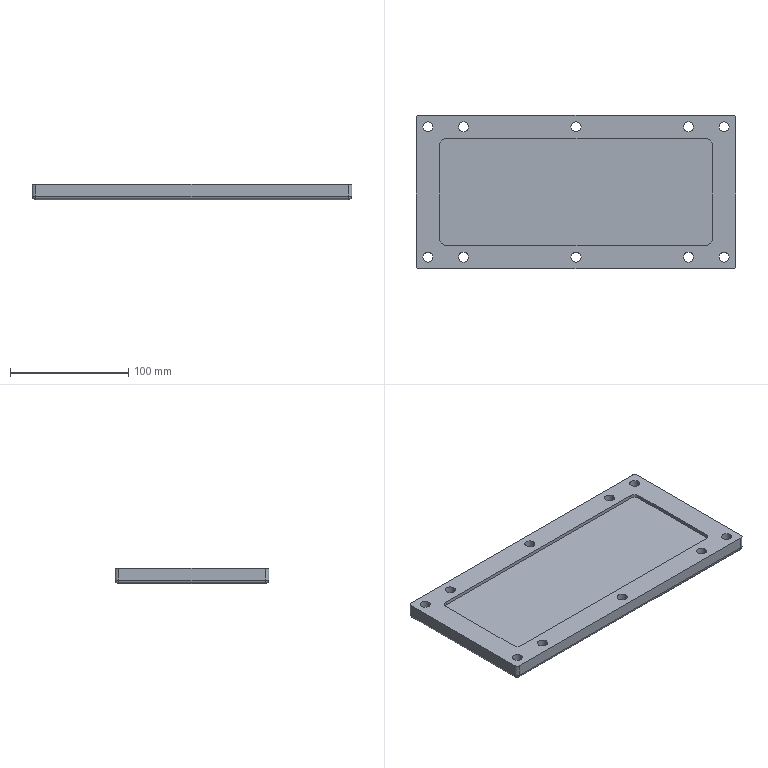Part | SolidWorks | features Extrusion 1, Fillet 1, ICE 1 | 1 solid | 47 faces | box 270 x 130 x 13 mm | volume 385260 mm3 | cylinder 32 | plane 11 | sphere 4 | commonest cylinder face diameters 8.5 x20 6 x8 10 x4
STEP:
#1=CARTESIAN_POINT('',(-129.25,-55.,13.));
#2=VERTEX_POINT('',#1);
#3=CARTESIAN_POINT('',(-120.75,-55.,13.));
#4=VERTEX_POINT('',#3);
#5=CARTESIAN_POINT('',(-125.,-55.,13.));
#6=DIRECTION('',(0.,0.,1.));
#7=DIRECTION('',(1.,0.,0.));
#8=AXIS2_PLACEMENT_3D('',#5,#6,#7);
#9=CIRCLE('',#8,4.25);
#10=EDGE_CURVE('',#2,#4,#9,.T.);
#11=ORIENTED_EDGE('',*,*,#10,.T.);
#12=CARTESIAN_POINT('',(-120.75,-55.,0.));
#13=VERTEX_POINT('',#12);
#14=CARTESIAN_POINT('',(-120.75,-55.,10.));
#15=DIRECTION('',(0.,0.,-1.));
#16=VECTOR('',#15,1000.);
#17=LINE('',#14,#16);
#18=EDGE_CURVE('',#4,#13,#17,.T.);
#19=ORIENTED_EDGE('',*,*,#18,.T.);
#20=CARTESIAN_POINT('',(-129.25,-55.,0.));
#21=VERTEX_POINT('',#20);
#22=CARTESIAN_POINT('',(-125.,-55.,0.));
#23=DIRECTION('',(0.,0.,1.));
#24=DIRECTION('',(1.,0.,0.));
#25=AXIS2_PLACEMENT_3D('',#22,#23,#24);
#26=CIRCLE('',#25,4.25);
#27=EDGE_CURVE('',#21,#13,#26,.T.);
#28=ORIENTED_EDGE('',*,*,#27,.F.);
#29=CARTESIAN_POINT('',(-129.25,-55.,10.));
#30=DIRECTION('',(0.,0.,-1.));
#31=VECTOR('',#30,1000.);
#32=LINE('',#29,#31);
#33=EDGE_CURVE('',#2,#21,#32,.T.);
#34=ORIENTED_EDGE('',*,*,#33,.F.);
#35=EDGE_LOOP('',(#11,#19,#28,#34));
#36=FACE_OUTER_BOUND('',#35,.T.);
#37=CARTESIAN_POINT('',(-125.,-55.,10.));
#38=DIRECTION('',(0.,0.,-1.));
#39=DIRECTION('',(-1.,0.,0.));
#40=AXIS2_PLACEMENT_3D('',#37,#38,#39);
#41=CYLINDRICAL_SURFACE('',#40,4.25);
#42=ADVANCED_FACE('',(#36),#41,.F.);
#43=CARTESIAN_POINT('',(-99.25,-55.,13.));
#44=VERTEX_POINT('',#43);
#45=CARTESIAN_POINT('',(-90.75,-55.,13.));
#46=VERTEX_POINT('',#45);
#47=CARTESIAN_POINT('',(-95.,-55.,13.));
#48=DIRECTION('',(0.,0.,1.));
#49=DIRECTION('',(1.,0.,0.));
#50=AXIS2_PLACEMENT_3D('',#47,#48,#49);
#51=CIRCLE('',#50,4.25);
#52=EDGE_CURVE('',#44,#46,#51,.T.);
#53=ORIENTED_EDGE('',*,*,#52,.T.);
#54=CARTESIAN_POINT('',(-90.75,-55.,0.));
#55=VERTEX_POINT('',#54);
#56=CARTESIAN_POINT('',(-90.75,-55.,10.));
#57=DIRECTION('',(0.,0.,-1.));
#58=VECTOR('',#57,1000.);
#59=LINE('',#56,#58);
#60=EDGE_CURVE('',#46,#55,#59,.T.);
#61=ORIENTED_EDGE('',*,*,#60,.T.);
#62=CARTESIAN_POINT('',(-99.25,-55.,0.));
#63=VERTEX_POINT('',#62);
#64=CARTESIAN_POINT('',(-95.,-55.,0.));
#65=DIRECTION('',(0.,0.,1.));
#66=DIRECTION('',(1.,0.,0.));
#67=AXIS2_PLACEMENT_3D('',#64,#65,#66);
#68=CIRCLE('',#67,4.25);
#69=EDGE_CURVE('',#63,#55,#68,.T.);
#70=ORIENTED_EDGE('',*,*,#69,.F.);
#71=CARTESIAN_POINT('',(-99.25,-55.,10.));
#72=DIRECTION('',(0.,0.,-1.));
#73=VECTOR('',#72,1000.);
#74=LINE('',#71,#73);
#75=EDGE_CURVE('',#44,#63,#74,.T.);
#76=ORIENTED_EDGE('',*,*,#75,.F.);
#77=EDGE_LOOP('',(#53,#61,#70,#76));
#78=FACE_OUTER_BOUND('',#77,.T.);
#79=CARTESIAN_POINT('',(-95.,-55.,10.));
#80=DIRECTION('',(0.,0.,-1.));
#81=DIRECTION('',(-1.,0.,0.));
#82=AXIS2_PLACEMENT_3D('',#79,#80,#81);
#83=CYLINDRICAL_SURFACE('',#82,4.25);
#84=ADVANCED_FACE('',(#78),#83,.F.);
#85=CARTESIAN_POINT('',(-4.25,-55.,13.));
#86=VERTEX_POINT('',#85);
#87=CARTESIAN_POINT('',(4.25,-55.,13.));
#88=VERTEX_POINT('',#87);
#89=CARTESIAN_POINT('',(0.,-55.,13.));
#90=DIRECTION('',(0.,0.,1.));
#91=DIRECTION('',(1.,0.,0.));
#92=AXIS2_PLACEMENT_3D('',#89,#90,#91);
#93=CIRCLE('',#92,4.25);
#94=EDGE_CURVE('',#86,#88,#93,.T.);
#95=ORIENTED_EDGE('',*,*,#94,.T.);
#96=CARTESIAN_POINT('',(4.25,-55.,0.));
#97=VERTEX_POINT('',#96);
#98=CARTESIAN_POINT('',(4.25,-55.,10.));
#99=DIRECTION('',(0.,0.,-1.));
#100=VECTOR('',#99,1000.);
#101=LINE('',#98,#100);
#102=EDGE_CURVE('',#88,#97,#101,.T.);
#103=ORIENTED_EDGE('',*,*,#102,.T.);
#104=CARTESIAN_POINT('',(-4.25,-55.,0.));
#105=VERTEX_POINT('',#104);
#106=CARTESIAN_POINT('',(0.,-55.,0.));
#107=DIRECTION('',(0.,0.,1.));
#108=DIRECTION('',(1.,0.,0.));
#109=AXIS2_PLACEMENT_3D('',#106,#107,#108);
#110=CIRCLE('',#109,4.25);
#111=EDGE_CURVE('',#105,#97,#110,.T.);
#112=ORIENTED_EDGE('',*,*,#111,.F.);
#113=CARTESIAN_POINT('',(-4.25,-55.,10.));
#114=DIRECTION('',(0.,0.,-1.));
#115=VECTOR('',#114,1000.);
#116=LINE('',#113,#115);
#117=EDGE_CURVE('',#86,#105,#116,.T.);
#118=ORIENTED_EDGE('',*,*,#117,.F.);
#119=EDGE_LOOP('',(#95,#103,#112,#118));
#120=FACE_OUTER_BOUND('',#119,.T.);
#121=CARTESIAN_POINT('',(0.,-55.,10.));
#122=DIRECTION('',(0.,0.,-1.));
#123=DIRECTION('',(-1.,0.,0.));
#124=AXIS2_PLACEMENT_3D('',#121,#122,#123);
#125=CYLINDRICAL_SURFACE('',#124,4.25);
#126=ADVANCED_FACE('',(#120),#125,.F.);
#127=CARTESIAN_POINT('',(90.75,-55.,13.));
#128=VERTEX_POINT('',#127);
#129=CARTESIAN_POINT('',(99.25,-55.,13.));
#130=VERTEX_POINT('',#129);
#131=CARTESIAN_POINT('',(95.,-55.,13.));
#132=DIRECTION('',(0.,0.,1.));
#133=DIRECTION('',(1.,0.,0.));
#134=AXIS2_PLACEMENT_3D('',#131,#132,#133);
#135=CIRCLE('',#134,4.25);
#136=EDGE_CURVE('',#128,#130,#135,.T.);
#137=ORIENTED_EDGE('',*,*,#136,.T.);
#138=CARTESIAN_POINT('',(99.25,-55.,0.));
#139=VERTEX_POINT('',#138);
#140=CARTESIAN_POINT('',(99.25,-55.,10.));
#141=DIRECTION('',(0.,0.,-1.));
#142=VECTOR('',#141,1000.);
#143=LINE('',#140,#142);
#144=EDGE_CURVE('',#130,#139,#143,.T.);
#145=ORIENTED_EDGE('',*,*,#144,.T.);
#146=CARTESIAN_POINT('',(90.75,-55.,0.));
#147=VERTEX_POINT('',#146);
#148=CARTESIAN_POINT('',(95.,-55.,0.));
#149=DIRECTION('',(0.,0.,1.));
#150=DIRECTION('',(1.,0.,0.));
#151=AXIS2_PLACEMENT_3D('',#148,#149,#150);
#152=CIRCLE('',#151,4.25);
#153=EDGE_CURVE('',#147,#139,#152,.T.);
#154=ORIENTED_EDGE('',*,*,#153,.F.);
#155=CARTESIAN_POINT('',(90.75,-55.,10.));
#156=DIRECTION('',(0.,0.,-1.));
#157=VECTOR('',#156,1000.);
#158=LINE('',#155,#157);
#159=EDGE_CURVE('',#128,#147,#158,.T.);
#160=ORIENTED_EDGE('',*,*,#159,.F.);
#161=EDGE_LOOP('',(#137,#145,#154,#160));
#162=FACE_OUTER_BOUND('',#161,.T.);
#163=CARTESIAN_POINT('',(95.,-55.,10.));
#164=DIRECTION('',(0.,0.,-1.));
#165=DIRECTION('',(-1.,0.,0.));
#166=AXIS2_PLACEMENT_3D('',#163,#164,#165);
#167=CYLINDRICAL_SURFACE('',#166,4.25);
#168=ADVANCED_FACE('',(#162),#167,.F.);
#169=CARTESIAN_POINT('',(120.75,-55.,13.));
#170=VERTEX_POINT('',#169);
#171=CARTESIAN_POINT('',(129.25,-55.,13.));
#172=VERTEX_POINT('',#171);
#173=CARTESIAN_POINT('',(125.,-55.,13.));
#174=DIRECTION('',(0.,0.,1.));
#175=DIRECTION('',(1.,0.,0.));
#176=AXIS2_PLACEMENT_3D('',#173,#174,#175);
#177=CIRCLE('',#176,4.25);
#178=EDGE_CURVE('',#170,#172,#177,.T.);
#179=ORIENTED_EDGE('',*,*,#178,.T.);
#180=CARTESIAN_POINT('',(129.25,-55.,0.));
#181=VERTEX_POINT('',#180);
#182=CARTESIAN_POINT('',(129.25,-55.,10.));
#183=DIRECTION('',(0.,0.,-1.));
#184=VECTOR('',#183,1000.);
#185=LINE('',#182,#184);
#186=EDGE_CURVE('',#172,#181,#185,.T.);
#187=ORIENTED_EDGE('',*,*,#186,.T.);
#188=CARTESIAN_POINT('',(120.75,-55.,0.));
#189=VERTEX_POINT('',#188);
#190=CARTESIAN_POINT('',(125.,-55.,0.));
#191=DIRECTION('',(0.,0.,1.));
#192=DIRECTION('',(1.,0.,0.));
#193=AXIS2_PLACEMENT_3D('',#190,#191,#192);
#194=CIRCLE('',#193,4.25);
#195=EDGE_CURVE('',#189,#181,#194,.T.);
#196=ORIENTED_EDGE('',*,*,#195,.F.);
#197=CARTESIAN_POINT('',(120.75,-55.,10.));
#198=DIRECTION('',(0.,0.,-1.));
#199=VECTOR('',#198,1000.);
#200=LINE('',#197,#199);
#201=EDGE_CURVE('',#170,#189,#200,.T.);
#202=ORIENTED_EDGE('',*,*,#201,.F.);
#203=EDGE_LOOP('',(#179,#187,#196,#202));
#204=FACE_OUTER_BOUND('',#203,.T.);
#205=CARTESIAN_POINT('',(125.,-55.,10.));
#206=DIRECTION('',(0.,0.,-1.));
#207=DIRECTION('',(-1.,0.,0.));
#208=AXIS2_PLACEMENT_3D('',#205,#206,#207);
#209=CYLINDRICAL_SURFACE('',#208,4.25);
#210=ADVANCED_FACE('',(#204),#209,.F.);
#211=CARTESIAN_POINT('',(120.75,55.,13.));
#212=VERTEX_POINT('',#211);
#213=CARTESIAN_POINT('',(129.25,55.,13.));
#214=VERTEX_POINT('',#213);
#215=CARTESIAN_POINT('',(125.,55.,13.));
#216=DIRECTION('',(0.,0.,1.));
#217=DIRECTION('',(1.,0.,0.));
#218=AXIS2_PLACEMENT_3D('',#215,#216,#217);
#219=CIRCLE('',#218,4.25);
#220=EDGE_CURVE('',#212,#214,#219,.T.);
#221=ORIENTED_EDGE('',*,*,#220,.T.);
#222=CARTESIAN_POINT('',(129.25,55.,0.));
#223=VERTEX_POINT('',#222);
#224=CARTESIAN_POINT('',(129.25,55.,10.));
#225=DIRECTION('',(0.,0.,-1.));
#226=VECTOR('',#225,1000.);
#227=LINE('',#224,#226);
#228=EDGE_CURVE('',#214,#223,#227,.T.);
#229=ORIENTED_EDGE('',*,*,#228,.T.);
#230=CARTESIAN_POINT('',(120.75,55.,0.));
#231=VERTEX_POINT('',#230);
#232=CARTESIAN_POINT('',(125.,55.,0.));
#233=DIRECTION('',(0.,0.,1.));
#234=DIRECTION('',(1.,0.,0.));
#235=AXIS2_PLACEMENT_3D('',#232,#233,#234);
#236=CIRCLE('',#235,4.25);
#237=EDGE_CURVE('',#231,#223,#236,.T.);
#238=ORIENTED_EDGE('',*,*,#237,.F.);
#239=CARTESIAN_POINT('',(120.75,55.,10.));
#240=DIRECTION('',(0.,0.,-1.));
#241=VECTOR('',#240,1000.);
#242=LINE('',#239,#241);
#243=EDGE_CURVE('',#212,#231,#242,.T.);
#244=ORIENTED_EDGE('',*,*,#243,.F.);
#245=EDGE_LOOP('',(#221,#229,#238,#244));
#246=FACE_OUTER_BOUND('',#245,.T.);
#247=CARTESIAN_POINT('',(125.,55.,10.));
#248=DIRECTION('',(0.,0.,-1.));
#249=DIRECTION('',(-1.,0.,0.));
#250=AXIS2_PLACEMENT_3D('',#247,#248,#249);
#251=CYLINDRICAL_SURFACE('',#250,4.25);
#252=ADVANCED_FACE('',(#246),#251,.F.);
#253=CARTESIAN_POINT('',(90.75,55.,13.));
#254=VERTEX_POINT('',#253);
#255=CARTESIAN_POINT('',(99.25,55.,13.));
#256=VERTEX_POINT('',#255);
#257=CARTESIAN_POINT('',(95.,55.,13.));
#258=DIRECTION('',(0.,0.,1.));
#259=DIRECTION('',(1.,0.,0.));
#260=AXIS2_PLACEMENT_3D('',#257,#258,#259);
#261=CIRCLE('',#260,4.25);
#262=EDGE_CURVE('',#254,#256,#261,.T.);
#263=ORIENTED_EDGE('',*,*,#262,.T.);
#264=CARTESIAN_POINT('',(99.25,55.,0.));
#265=VERTEX_POINT('',#264);
#266=CARTESIAN_POINT('',(99.25,55.,10.));
#267=DIRECTION('',(0.,0.,-1.));
#268=VECTOR('',#267,1000.);
#269=LINE('',#266,#268);
#270=EDGE_CURVE('',#256,#265,#269,.T.);
#271=ORIENTED_EDGE('',*,*,#270,.T.);
#272=CARTESIAN_POINT('',(90.75,55.,0.));
#273=VERTEX_POINT('',#272);
#274=CARTESIAN_POINT('',(95.,55.,0.));
#275=DIRECTION('',(0.,0.,1.));
#276=DIRECTION('',(1.,0.,0.));
#277=AXIS2_PLACEMENT_3D('',#274,#275,#276);
#278=CIRCLE('',#277,4.25);
#279=EDGE_CURVE('',#273,#265,#278,.T.);
#280=ORIENTED_EDGE('',*,*,#279,.F.);
#281=CARTESIAN_POINT('',(90.75,55.,10.));
#282=DIRECTION('',(0.,0.,-1.));
#283=VECTOR('',#282,1000.);
#284=LINE('',#281,#283);
#285=EDGE_CURVE('',#254,#273,#284,.T.);
#286=ORIENTED_EDGE('',*,*,#285,.F.);
#287=EDGE_LOOP('',(#263,#271,#280,#286));
#288=FACE_OUTER_BOUND('',#287,.T.);
#289=CARTESIAN_POINT('',(95.,55.,10.));
#290=DIRECTION('',(0.,0.,-1.));
#291=DIRECTION('',(-1.,0.,0.));
#292=AXIS2_PLACEMENT_3D('',#289,#290,#291);
#293=CYLINDRICAL_SURFACE('',#292,4.25);
#294=ADVANCED_FACE('',(#288),#293,.F.);
#295=CARTESIAN_POINT('',(-4.25,55.,13.));
#296=VERTEX_POINT('',#295);
#297=CARTESIAN_POINT('',(4.25,55.,13.));
#298=VERTEX_POINT('',#297);
#299=CARTESIAN_POINT('',(0.,55.,13.));
#300=DIRECTION('',(0.,0.,1.));
#301=DIRECTION('',(1.,0.,0.));
#302=AXIS2_PLACEMENT_3D('',#299,#300,#301);
#303=CIRCLE('',#302,4.25);
#304=EDGE_CURVE('',#296,#298,#303,.T.);
#305=ORIENTED_EDGE('',*,*,#304,.T.);
#306=CARTESIAN_POINT('',(4.25,55.,0.));
#307=VERTEX_POINT('',#306);
#308=CARTESIAN_POINT('',(4.25,55.,10.));
#309=DIRECTION('',(0.,0.,-1.));
#310=VECTOR('',#309,1000.);
#311=LINE('',#308,#310);
#312=EDGE_CURVE('',#298,#307,#311,.T.);
#313=ORIENTED_EDGE('',*,*,#312,.T.);
#314=CARTESIAN_POINT('',(-4.25,55.,0.));
#315=VERTEX_POINT('',#314);
#316=CARTESIAN_POINT('',(0.,55.,0.));
#317=DIRECTION('',(0.,0.,1.));
#318=DIRECTION('',(1.,0.,0.));
#319=AXIS2_PLACEMENT_3D('',#316,#317,#318);
#320=CIRCLE('',#319,4.25);
#321=EDGE_CURVE('',#315,#307,#320,.T.);
#322=ORIENTED_EDGE('',*,*,#321,.F.);
#323=CARTESIAN_POINT('',(-4.25,55.,10.));
#324=DIRECTION('',(0.,0.,-1.));
#325=VECTOR('',#324,1000.);
#326=LINE('',#323,#325);
#327=EDGE_CURVE('',#296,#315,#326,.T.);
#328=ORIENTED_EDGE('',*,*,#327,.F.);
#329=EDGE_LOOP('',(#305,#313,#322,#328));
#330=FACE_OUTER_BOUND('',#329,.T.);
#331=CARTESIAN_POINT('',(0.,55.,10.));
#332=DIRECTION('',(0.,0.,-1.));
#333=DIRECTION('',(-1.,0.,0.));
#334=AXIS2_PLACEMENT_3D('',#331,#332,#333);
#335=CYLINDRICAL_SURFACE('',#334,4.25);
#336=ADVANCED_FACE('',(#330),#335,.F.);
#337=CARTESIAN_POINT('',(-99.25,55.,13.));
#338=VERTEX_POINT('',#337);
#339=CARTESIAN_POINT('',(-90.75,55.,13.));
#340=VERTEX_POINT('',#339);
#341=CARTESIAN_POINT('',(-95.,55.,13.));
#342=DIRECTION('',(0.,0.,1.));
#343=DIRECTION('',(1.,0.,0.));
#344=AXIS2_PLACEMENT_3D('',#341,#342,#343);
#345=CIRCLE('',#344,4.25);
#346=EDGE_CURVE('',#338,#340,#345,.T.);
#347=ORIENTED_EDGE('',*,*,#346,.T.);
#348=CARTESIAN_POINT('',(-90.75,55.,0.));
#349=VERTEX_POINT('',#348);
#350=CARTESIAN_POINT('',(-90.75,55.,10.));
#351=DIRECTION('',(0.,0.,-1.));
#352=VECTOR('',#351,1000.);
#353=LINE('',#350,#352);
#354=EDGE_CURVE('',#340,#349,#353,.T.);
#355=ORIENTED_EDGE('',*,*,#354,.T.);
#356=CARTESIAN_POINT('',(-99.25,55.,0.));
#357=VERTEX_POINT('',#356);
#358=CARTESIAN_POINT('',(-95.,55.,0.));
#359=DIRECTION('',(0.,0.,1.));
#360=DIRECTION('',(1.,0.,0.));
#361=AXIS2_PLACEMENT_3D('',#358,#359,#360);
#362=CIRCLE('',#361,4.25);
#363=EDGE_CURVE('',#357,#349,#362,.T.);
#364=ORIENTED_EDGE('',*,*,#363,.F.);
#365=CARTESIAN_POINT('',(-99.25,55.,10.));
#366=DIRECTION('',(0.,0.,-1.));
#367=VECTOR('',#366,1000.);
#368=LINE('',#365,#367);
#369=EDGE_CURVE('',#338,#357,#368,.T.);
#370=ORIENTED_EDGE('',*,*,#369,.F.);
#371=EDGE_LOOP('',(#347,#355,#364,#370));
#372=FACE_OUTER_BOUND('',#371,.T.);
#373=CARTESIAN_POINT('',(-95.,55.,10.));
#374=DIRECTION('',(0.,0.,-1.));
#375=DIRECTION('',(-1.,0.,0.));
#376=AXIS2_PLACEMENT_3D('',#373,#374,#375);
#377=CYLINDRICAL_SURFACE('',#376,4.25);
#378=ADVANCED_FACE('',(#372),#377,.F.);
#379=CARTESIAN_POINT('',(-129.25,55.,13.));
#380=VERTEX_POINT('',#379);
#381=CARTESIAN_POINT('',(-120.75,55.,13.));
#382=VERTEX_POINT('',#381);
#383=CARTESIAN_POINT('',(-125.,55.,13.));
#384=DIRECTION('',(0.,0.,1.));
#385=DIRECTION('',(1.,0.,0.));
#386=AXIS2_PLACEMENT_3D('',#383,#384,#385);
#387=CIRCLE('',#386,4.25);
#388=EDGE_CURVE('',#380,#382,#387,.T.);
#389=ORIENTED_EDGE('',*,*,#388,.T.);
#390=CARTESIAN_POINT('',(-120.75,55.,0.));
#391=VERTEX_POINT('',#390);
#392=CARTESIAN_POINT('',(-120.75,55.,10.));
#393=DIRECTION('',(0.,0.,-1.));
#394=VECTOR('',#393,1000.);
#395=LINE('',#392,#394);
#396=EDGE_CURVE('',#382,#391,#395,.T.);
#397=ORIENTED_EDGE('',*,*,#396,.T.);
#398=CARTESIAN_POINT('',(-129.25,55.,0.));
#399=VERTEX_POINT('',#398);
#400=CARTESIAN_POINT('',(-125.,55.,0.));
#401=DIRECTION('',(0.,0.,1.));
#402=DIRECTION('',(1.,0.,0.));
#403=AXIS2_PLACEMENT_3D('',#400,#401,#402);
#404=CIRCLE('',#403,4.25);
#405=EDGE_CURVE('',#399,#391,#404,.T.);
#406=ORIENTED_EDGE('',*,*,#405,.F.);
#407=CARTESIAN_POINT('',(-129.25,55.,10.));
#408=DIRECTION('',(0.,0.,-1.));
#409=VECTOR('',#408,1000.);
#410=LINE('',#407,#409);
#411=EDGE_CURVE('',#380,#399,#410,.T.);
#412=ORIENTED_EDGE('',*,*,#411,.F.);
#413=EDGE_LOOP('',(#389,#397,#406,#412));
#414=FACE_OUTER_BOUND('',#413,.T.);
#415=CARTESIAN_POINT('',(-125.,55.,10.));
#416=DIRECTION('',(0.,0.,-1.));
#417=DIRECTION('',(-1.,0.,0.));
#418=AXIS2_PLACEMENT_3D('',#415,#416,#417);
#419=CYLINDRICAL_SURFACE('',#418,4.25);
#420=ADVANCED_FACE('',(#414),#419,.F.);
#421=CARTESIAN_POINT('',(132.,62.,0.));
#422=VERTEX_POINT('',#421);
#423=CARTESIAN_POINT('',(132.,-62.,0.));
#424=VERTEX_POINT('',#423);
#425=CARTESIAN_POINT('',(132.,-62.,0.));
#426=DIRECTION('',(0.,-1.,0.));
#427=VECTOR('',#426,1000.);
#428=LINE('',#425,#427);
#429=EDGE_CURVE('',#422,#424,#428,.T.);
#430=ORIENTED_EDGE('',*,*,#429,.T.);
#431=CARTESIAN_POINT('',(-132.,-62.,0.));
#432=VERTEX_POINT('',#431);
#433=CARTESIAN_POINT('',(-132.,-62.,0.));
#434=DIRECTION('',(-1.,0.,0.));
#435=VECTOR('',#434,1000.);
#436=LINE('',#433,#435);
#437=EDGE_CURVE('',#424,#432,#436,.T.);
#438=ORIENTED_EDGE('',*,*,#437,.T.);
#439=CARTESIAN_POINT('',(-132.,62.,0.));
#440=VERTEX_POINT('',#439);
#441=CARTESIAN_POINT('',(-132.,62.,0.));
#442=DIRECTION('',(0.,1.,0.));
#443=VECTOR('',#442,1000.);
#444=LINE('',#441,#443);
#445=EDGE_CURVE('',#432,#440,#444,.T.);
#446=ORIENTED_EDGE('',*,*,#445,.T.);
#447=CARTESIAN_POINT('',(132.,62.,0.));
#448=DIRECTION('',(1.,0.,0.));
#449=VECTOR('',#448,1000.);
#450=LINE('',#447,#449);
#451=EDGE_CURVE('',#440,#422,#450,.T.);
#452=ORIENTED_EDGE('',*,*,#451,.T.);
#453=EDGE_LOOP('',(#430,#438,#446,#452));
#454=FACE_OUTER_BOUND('',#453,.T.);
#455=ORIENTED_EDGE('',*,*,#69,.T.);
#456=CARTESIAN_POINT('',(-95.,-55.,0.));
#457=DIRECTION('',(0.,0.,1.));
#458=DIRECTION('',(1.,0.,0.));
#459=AXIS2_PLACEMENT_3D('',#456,#457,#458);
#460=CIRCLE('',#459,4.25);
#461=EDGE_CURVE('',#55,#63,#460,.T.);
#462=ORIENTED_EDGE('',*,*,#461,.T.);
#463=EDGE_LOOP('',(#455,#462));
#464=FACE_BOUND('',#463,.T.);
#465=ORIENTED_EDGE('',*,*,#153,.T.);
#466=CARTESIAN_POINT('',(95.,-55.,0.));
#467=DIRECTION('',(0.,0.,1.));
#468=DIRECTION('',(1.,0.,0.));
#469=AXIS2_PLACEMENT_3D('',#466,#467,#468);
#470=CIRCLE('',#469,4.25);
#471=EDGE_CURVE('',#139,#147,#470,.T.);
#472=ORIENTED_EDGE('',*,*,#471,.T.);
#473=EDGE_LOOP('',(#465,#472));
#474=FACE_BOUND('',#473,.T.);
#475=ORIENTED_EDGE('',*,*,#237,.T.);
#476=CARTESIAN_POINT('',(125.,55.,0.));
#477=DIRECTION('',(0.,0.,1.));
#478=DIRECTION('',(1.,0.,0.));
#479=AXIS2_PLACEMENT_3D('',#476,#477,#478);
#480=CIRCLE('',#479,4.25);
#481=EDGE_CURVE('',#223,#231,#480,.T.);
#482=ORIENTED_EDGE('',*,*,#481,.T.);
#483=EDGE_LOOP('',(#475,#482));
#484=FACE_BOUND('',#483,.T.);
#485=ORIENTED_EDGE('',*,*,#321,.T.);
#486=CARTESIAN_POINT('',(0.,55.,0.));
#487=DIRECTION('',(0.,0.,1.));
#488=DIRECTION('',(1.,0.,0.));
#489=AXIS2_PLACEMENT_3D('',#486,#487,#488);
#490=CIRCLE('',#489,4.25);
#491=EDGE_CURVE('',#307,#315,#490,.T.);
#492=ORIENTED_EDGE('',*,*,#491,.T.);
#493=EDGE_LOOP('',(#485,#492));
#494=FACE_BOUND('',#493,.T.);
#495=ORIENTED_EDGE('',*,*,#405,.T.);
#496=CARTESIAN_POINT('',(-125.,55.,0.));
#497=DIRECTION('',(0.,0.,1.));
#498=DIRECTION('',(1.,0.,0.));
#499=AXIS2_PLACEMENT_3D('',#496,#497,#498);
#500=CIRCLE('',#499,4.25);
#501=EDGE_CURVE('',#391,#399,#500,.T.);
#502=ORIENTED_EDGE('',*,*,#501,.T.);
#503=EDGE_LOOP('',(#495,#502));
#504=FACE_BOUND('',#503,.T.);
#505=ORIENTED_EDGE('',*,*,#363,.T.);
#506=CARTESIAN_POINT('',(-95.,55.,0.));
#507=DIRECTION('',(0.,0.,1.));
#508=DIRECTION('',(1.,0.,0.));
#509=AXIS2_PLACEMENT_3D('',#506,#507,#508);
#510=CIRCLE('',#509,4.25);
#511=EDGE_CURVE('',#349,#357,#510,.T.);
#512=ORIENTED_EDGE('',*,*,#511,.T.);
#513=EDGE_LOOP('',(#505,#512));
#514=FACE_BOUND('',#513,.T.);
#515=ORIENTED_EDGE('',*,*,#279,.T.);
#516=CARTESIAN_POINT('',(95.,55.,0.));
#517=DIRECTION('',(0.,0.,1.));
#518=DIRECTION('',(1.,0.,0.));
#519=AXIS2_PLACEMENT_3D('',#516,#517,#518);
#520=CIRCLE('',#519,4.25);
#521=EDGE_CURVE('',#265,#273,#520,.T.);
#522=ORIENTED_EDGE('',*,*,#521,.T.);
#523=EDGE_LOOP('',(#515,#522));
#524=FACE_BOUND('',#523,.T.);
#525=ORIENTED_EDGE('',*,*,#195,.T.);
#526=CARTESIAN_POINT('',(125.,-55.,0.));
#527=DIRECTION('',(0.,0.,1.));
#528=DIRECTION('',(1.,0.,0.));
#529=AXIS2_PLACEMENT_3D('',#526,#527,#528);
#530=CIRCLE('',#529,4.25);
#531=EDGE_CURVE('',#181,#189,#530,.T.);
#532=ORIENTED_EDGE('',*,*,#531,.T.);
#533=EDGE_LOOP('',(#525,#532));
#534=FACE_BOUND('',#533,.T.);
#535=ORIENTED_EDGE('',*,*,#111,.T.);
#536=CARTESIAN_POINT('',(0.,-55.,0.));
#537=DIRECTION('',(0.,0.,1.));
#538=DIRECTION('',(1.,0.,0.));
#539=AXIS2_PLACEMENT_3D('',#536,#537,#538);
#540=CIRCLE('',#539,4.25);
#541=EDGE_CURVE('',#97,#105,#540,.T.);
#542=ORIENTED_EDGE('',*,*,#541,.T.);
#543=EDGE_LOOP('',(#535,#542));
#544=FACE_BOUND('',#543,.T.);
#545=ORIENTED_EDGE('',*,*,#27,.T.);
#546=CARTESIAN_POINT('',(-125.,-55.,0.));
#547=DIRECTION('',(0.,0.,1.));
#548=DIRECTION('',(1.,0.,0.));
#549=AXIS2_PLACEMENT_3D('',#546,#547,#548);
#550=CIRCLE('',#549,4.25);
#551=EDGE_CURVE('',#13,#21,#550,.T.);
#552=ORIENTED_EDGE('',*,*,#551,.T.);
#553=EDGE_LOOP('',(#545,#552));
#554=FACE_BOUND('',#553,.T.);
#555=CARTESIAN_POINT('',(132.,62.,0.));
#556=DIRECTION('',(0.,0.,-1.));
#557=DIRECTION('',(-1.,0.,0.));
#558=AXIS2_PLACEMENT_3D('',#555,#556,#557);
#559=PLANE('',#558);
#560=ADVANCED_FACE('',(#454,#464,#474,#484,#494,#504,#514,#524,#534,#544,#554),#559,.T.);
#561=CARTESIAN_POINT('',(135.,62.,13.));
#562=VERTEX_POINT('',#561);
#563=CARTESIAN_POINT('',(135.,62.,3.));
#564=VERTEX_POINT('',#563);
#565=CARTESIAN_POINT('',(135.,62.,10.));
#566=DIRECTION('',(0.,0.,-1.));
#567=VECTOR('',#566,1000.);
#568=LINE('',#565,#567);
#569=EDGE_CURVE('',#562,#564,#568,.T.);
#570=ORIENTED_EDGE('',*,*,#569,.T.);
#571=CARTESIAN_POINT('',(132.,65.,3.));
#572=VERTEX_POINT('',#571);
#573=CARTESIAN_POINT('',(132.,62.,3.));
#574=DIRECTION('',(0.,0.,1.));
#575=DIRECTION('',(-1.,0.,0.));
#576=AXIS2_PLACEMENT_3D('',#573,#574,#575);
#577=CIRCLE('',#576,3.);
#578=EDGE_CURVE('',#564,#572,#577,.T.);
#579=ORIENTED_EDGE('',*,*,#578,.T.);
#580=CARTESIAN_POINT('',(132.,65.,13.));
#581=VERTEX_POINT('',#580);
#582=CARTESIAN_POINT('',(132.,65.,10.));
#583=DIRECTION('',(0.,0.,-1.));
#584=VECTOR('',#583,1000.);
#585=LINE('',#582,#584);
#586=EDGE_CURVE('',#581,#572,#585,.T.);
#587=ORIENTED_EDGE('',*,*,#586,.F.);
#588=CARTESIAN_POINT('',(132.,62.,13.));
#589=DIRECTION('',(0.,0.,1.));
#590=DIRECTION('',(1.,0.,0.));
#591=AXIS2_PLACEMENT_3D('',#588,#589,#590);
#592=CIRCLE('',#591,3.);
#593=EDGE_CURVE('',#562,#581,#592,.T.);
#594=ORIENTED_EDGE('',*,*,#593,.F.);
#595=EDGE_LOOP('',(#570,#579,#587,#594));
#596=FACE_OUTER_BOUND('',#595,.T.);
#597=CARTESIAN_POINT('',(132.,62.,10.));
#598=DIRECTION('',(0.,0.,-1.));
#599=DIRECTION('',(-1.,0.,0.));
#600=AXIS2_PLACEMENT_3D('',#597,#598,#599);
#601=CYLINDRICAL_SURFACE('',#600,3.);
#602=ADVANCED_FACE('',(#596),#601,.T.);
#603=ORIENTED_EDGE('',*,*,#586,.T.);
#604=CARTESIAN_POINT('',(-132.,65.,3.));
#605=VERTEX_POINT('',#604);
#606=CARTESIAN_POINT('',(-132.,65.,3.));
#607=DIRECTION('',(-1.,0.,0.));
#608=VECTOR('',#607,1000.);
#609=LINE('',#606,#608);
#610=EDGE_CURVE('',#572,#605,#609,.T.);
#611=ORIENTED_EDGE('',*,*,#610,.T.);
#612=CARTESIAN_POINT('',(-132.,65.,13.));
#613=VERTEX_POINT('',#612);
#614=CARTESIAN_POINT('',(-132.,65.,10.));
#615=DIRECTION('',(0.,0.,-1.));
#616=VECTOR('',#615,1000.);
#617=LINE('',#614,#616);
#618=EDGE_CURVE('',#613,#605,#617,.T.);
#619=ORIENTED_EDGE('',*,*,#618,.F.);
#620=CARTESIAN_POINT('',(132.,65.,13.));
#621=DIRECTION('',(-1.,0.,0.));
#622=VECTOR('',#621,1000.);
#623=LINE('',#620,#622);
#624=EDGE_CURVE('',#581,#613,#623,.T.);
#625=ORIENTED_EDGE('',*,*,#624,.F.);
#626=EDGE_LOOP('',(#603,#611,#619,#625));
#627=FACE_OUTER_BOUND('',#626,.T.);
#628=CARTESIAN_POINT('',(-132.,65.,10.));
#629=DIRECTION('',(0.,-1.,0.));
#630=DIRECTION('',(0.,0.,-1.));
#631=AXIS2_PLACEMENT_3D('',#628,#629,#630);
#632=PLANE('',#631);
#633=ADVANCED_FACE('',(#627),#632,.F.);
#634=ORIENTED_EDGE('',*,*,#618,.T.);
#635=CARTESIAN_POINT('',(-135.,62.,3.));
#636=VERTEX_POINT('',#635);
#637=CARTESIAN_POINT('',(-132.,62.,3.));
#638=DIRECTION('',(0.,0.,1.));
#639=DIRECTION('',(-1.,0.,0.));
#640=AXIS2_PLACEMENT_3D('',#637,#638,#639);
#641=CIRCLE('',#640,3.);
#642=EDGE_CURVE('',#605,#636,#641,.T.);
#643=ORIENTED_EDGE('',*,*,#642,.T.);
#644=CARTESIAN_POINT('',(-135.,62.,13.));
#645=VERTEX_POINT('',#644);
#646=CARTESIAN_POINT('',(-135.,62.,10.));
#647=DIRECTION('',(0.,0.,-1.));
#648=VECTOR('',#647,1000.);
#649=LINE('',#646,#648);
#650=EDGE_CURVE('',#645,#636,#649,.T.);
#651=ORIENTED_EDGE('',*,*,#650,.F.);
#652=CARTESIAN_POINT('',(-132.,62.,13.));
#653=DIRECTION('',(0.,0.,1.));
#654=DIRECTION('',(1.,0.,0.));
#655=AXIS2_PLACEMENT_3D('',#652,#653,#654);
#656=CIRCLE('',#655,3.);
#657=EDGE_CURVE('',#613,#645,#656,.T.);
#658=ORIENTED_EDGE('',*,*,#657,.F.);
#659=EDGE_LOOP('',(#634,#643,#651,#658));
#660=FACE_OUTER_BOUND('',#659,.T.);
#661=CARTESIAN_POINT('',(-132.,62.,10.));
#662=DIRECTION('',(0.,0.,-1.));
#663=DIRECTION('',(-1.,0.,0.));
#664=AXIS2_PLACEMENT_3D('',#661,#662,#663);
#665=CYLINDRICAL_SURFACE('',#664,3.);
#666=ADVANCED_FACE('',(#660),#665,.T.);
#667=ORIENTED_EDGE('',*,*,#650,.T.);
#668=CARTESIAN_POINT('',(-135.,-62.,3.));
#669=VERTEX_POINT('',#668);
#670=CARTESIAN_POINT('',(-135.,-62.,3.));
#671=DIRECTION('',(0.,-1.,0.));
#672=VECTOR('',#671,1000.);
#673=LINE('',#670,#672);
#674=EDGE_CURVE('',#636,#669,#673,.T.);
#675=ORIENTED_EDGE('',*,*,#674,.T.);
#676=CARTESIAN_POINT('',(-135.,-62.,13.));
#677=VERTEX_POINT('',#676);
#678=CARTESIAN_POINT('',(-135.,-62.,10.));
#679=DIRECTION('',(0.,0.,-1.));
#680=VECTOR('',#679,1000.);
#681=LINE('',#678,#680);
#682=EDGE_CURVE('',#677,#669,#681,.T.);
#683=ORIENTED_EDGE('',*,*,#682,.F.);
#684=CARTESIAN_POINT('',(-135.,62.,13.));
#685=DIRECTION('',(0.,-1.,0.));
#686=VECTOR('',#685,1000.);
#687=LINE('',#684,#686);
#688=EDGE_CURVE('',#645,#677,#687,.T.);
#689=ORIENTED_EDGE('',*,*,#688,.F.);
#690=EDGE_LOOP('',(#667,#675,#683,#689));
#691=FACE_OUTER_BOUND('',#690,.T.);
#692=CARTESIAN_POINT('',(-135.,-62.,10.));
#693=DIRECTION('',(1.,0.,0.));
#694=DIRECTION('',(0.,0.,-1.));
#695=AXIS2_PLACEMENT_3D('',#692,#693,#694);
#696=PLANE('',#695);
#697=ADVANCED_FACE('',(#691),#696,.F.);
#698=ORIENTED_EDGE('',*,*,#682,.T.);
#699=CARTESIAN_POINT('',(-132.,-65.,3.));
#700=VERTEX_POINT('',#699);
#701=CARTESIAN_POINT('',(-132.,-62.,3.));
#702=DIRECTION('',(0.,0.,1.));
#703=DIRECTION('',(-1.,0.,0.));
#704=AXIS2_PLACEMENT_3D('',#701,#702,#703);
#705=CIRCLE('',#704,3.);
#706=EDGE_CURVE('',#669,#700,#705,.T.);
#707=ORIENTED_EDGE('',*,*,#706,.T.);
#708=CARTESIAN_POINT('',(-132.,-65.,13.));
#709=VERTEX_POINT('',#708);
#710=CARTESIAN_POINT('',(-132.,-65.,10.));
#711=DIRECTION('',(0.,0.,-1.));
#712=VECTOR('',#711,1000.);
#713=LINE('',#710,#712);
#714=EDGE_CURVE('',#709,#700,#713,.T.);
#715=ORIENTED_EDGE('',*,*,#714,.F.);
#716=CARTESIAN_POINT('',(-132.,-62.,13.));
#717=DIRECTION('',(0.,0.,1.));
#718=DIRECTION('',(1.,0.,0.));
#719=AXIS2_PLACEMENT_3D('',#716,#717,#718);
#720=CIRCLE('',#719,3.);
#721=EDGE_CURVE('',#677,#709,#720,.T.);
#722=ORIENTED_EDGE('',*,*,#721,.F.);
#723=EDGE_LOOP('',(#698,#707,#715,#722));
#724=FACE_OUTER_BOUND('',#723,.T.);
#725=CARTESIAN_POINT('',(-132.,-62.,10.));
#726=DIRECTION('',(0.,0.,-1.));
#727=DIRECTION('',(-1.,0.,0.));
#728=AXIS2_PLACEMENT_3D('',#725,#726,#727);
#729=CYLINDRICAL_SURFACE('',#728,3.);
#730=ADVANCED_FACE('',(#724),#729,.T.);
#731=ORIENTED_EDGE('',*,*,#714,.T.);
#732=CARTESIAN_POINT('',(132.,-65.,3.));
#733=VERTEX_POINT('',#732);
#734=CARTESIAN_POINT('',(132.,-65.,3.));
#735=DIRECTION('',(1.,0.,0.));
#736=VECTOR('',#735,1000.);
#737=LINE('',#734,#736);
#738=EDGE_CURVE('',#700,#733,#737,.T.);
#739=ORIENTED_EDGE('',*,*,#738,.T.);
#740=CARTESIAN_POINT('',(132.,-65.,13.));
#741=VERTEX_POINT('',#740);
#742=CARTESIAN_POINT('',(132.,-65.,10.));
#743=DIRECTION('',(0.,0.,-1.));
#744=VECTOR('',#743,1000.);
#745=LINE('',#742,#744);
#746=EDGE_CURVE('',#741,#733,#745,.T.);
#747=ORIENTED_EDGE('',*,*,#746,.F.);
#748=CARTESIAN_POINT('',(-132.,-65.,13.));
#749=DIRECTION('',(1.,0.,0.));
#750=VECTOR('',#749,1000.);
#751=LINE('',#748,#750);
#752=EDGE_CURVE('',#709,#741,#751,.T.);
#753=ORIENTED_EDGE('',*,*,#752,.F.);
#754=EDGE_LOOP('',(#731,#739,#747,#753));
#755=FACE_OUTER_BOUND('',#754,.T.);
#756=CARTESIAN_POINT('',(-132.,-65.,10.));
#757=DIRECTION('',(0.,1.,0.));
#758=DIRECTION('',(0.,0.,1.));
#759=AXIS2_PLACEMENT_3D('',#756,#757,#758);
#760=PLANE('',#759);
#761=ADVANCED_FACE('',(#755),#760,.F.);
#762=ORIENTED_EDGE('',*,*,#746,.T.);
#763=CARTESIAN_POINT('',(135.,-62.,3.));
#764=VERTEX_POINT('',#763);
#765=CARTESIAN_POINT('',(132.,-62.,3.));
#766=DIRECTION('',(0.,0.,1.));
#767=DIRECTION('',(-1.,0.,0.));
#768=AXIS2_PLACEMENT_3D('',#765,#766,#767);
#769=CIRCLE('',#768,3.);
#770=EDGE_CURVE('',#733,#764,#769,.T.);
#771=ORIENTED_EDGE('',*,*,#770,.T.);
#772=CARTESIAN_POINT('',(135.,-62.,13.));
#773=VERTEX_POINT('',#772);
#774=CARTESIAN_POINT('',(135.,-62.,10.));
#775=DIRECTION('',(0.,0.,-1.));
#776=VECTOR('',#775,1000.);
#777=LINE('',#774,#776);
#778=EDGE_CURVE('',#773,#764,#777,.T.);
#779=ORIENTED_EDGE('',*,*,#778,.F.);
#780=CARTESIAN_POINT('',(132.,-62.,13.));
#781=DIRECTION('',(0.,0.,1.));
#782=DIRECTION('',(1.,0.,0.));
#783=AXIS2_PLACEMENT_3D('',#780,#781,#782);
#784=CIRCLE('',#783,3.);
#785=EDGE_CURVE('',#741,#773,#784,.T.);
#786=ORIENTED_EDGE('',*,*,#785,.F.);
#787=EDGE_LOOP('',(#762,#771,#779,#786));
#788=FACE_OUTER_BOUND('',#787,.T.);
#789=CARTESIAN_POINT('',(132.,-62.,10.));
#790=DIRECTION('',(0.,0.,-1.));
#791=DIRECTION('',(-1.,0.,0.));
#792=AXIS2_PLACEMENT_3D('',#789,#790,#791);
#793=CYLINDRICAL_SURFACE('',#792,3.);
#794=ADVANCED_FACE('',(#788),#793,.T.);
#795=ORIENTED_EDGE('',*,*,#778,.T.);
#796=CARTESIAN_POINT('',(135.,62.,3.));
#797=DIRECTION('',(0.,1.,0.));
#798=VECTOR('',#797,1000.);
#799=LINE('',#796,#798);
#800=EDGE_CURVE('',#764,#564,#799,.T.);
#801=ORIENTED_EDGE('',*,*,#800,.T.);
#802=ORIENTED_EDGE('',*,*,#569,.F.);
#803=CARTESIAN_POINT('',(135.,-62.,13.));
#804=DIRECTION('',(0.,1.,0.));
#805=VECTOR('',#804,1000.);
#806=LINE('',#803,#805);
#807=EDGE_CURVE('',#773,#562,#806,.T.);
#808=ORIENTED_EDGE('',*,*,#807,.F.);
#809=EDGE_LOOP('',(#795,#801,#802,#808));
#810=FACE_OUTER_BOUND('',#809,.T.);
#811=CARTESIAN_POINT('',(135.,-62.,10.));
#812=DIRECTION('',(-1.,0.,0.));
#813=DIRECTION('',(0.,0.,1.));
#814=AXIS2_PLACEMENT_3D('',#811,#812,#813);
#815=PLANE('',#814);
#816=ADVANCED_FACE('',(#810),#815,.F.);
#817=ORIENTED_EDGE('',*,*,#396,.F.);
#818=CARTESIAN_POINT('',(-125.,55.,13.));
#819=DIRECTION('',(0.,0.,1.));
#820=DIRECTION('',(1.,0.,0.));
#821=AXIS2_PLACEMENT_3D('',#818,#819,#820);
#822=CIRCLE('',#821,4.25);
#823=EDGE_CURVE('',#382,#380,#822,.T.);
#824=ORIENTED_EDGE('',*,*,#823,.T.);
#825=ORIENTED_EDGE('',*,*,#411,.T.);
#826=ORIENTED_EDGE('',*,*,#501,.F.);
#827=EDGE_LOOP('',(#817,#824,#825,#826));
#828=FACE_OUTER_BOUND('',#827,.T.);
#829=CARTESIAN_POINT('',(-125.,55.,10.));
#830=DIRECTION('',(0.,0.,-1.));
#831=DIRECTION('',(-1.,0.,0.));
#832=AXIS2_PLACEMENT_3D('',#829,#830,#831);
#833=CYLINDRICAL_SURFACE('',#832,4.25);
#834=ADVANCED_FACE('',(#828),#833,.F.);
#835=ORIENTED_EDGE('',*,*,#354,.F.);
#836=CARTESIAN_POINT('',(-95.,55.,13.));
#837=DIRECTION('',(0.,0.,1.));
#838=DIRECTION('',(1.,0.,0.));
#839=AXIS2_PLACEMENT_3D('',#836,#837,#838);
#840=CIRCLE('',#839,4.25);
#841=EDGE_CURVE('',#340,#338,#840,.T.);
#842=ORIENTED_EDGE('',*,*,#841,.T.);
#843=ORIENTED_EDGE('',*,*,#369,.T.);
#844=ORIENTED_EDGE('',*,*,#511,.F.);
#845=EDGE_LOOP('',(#835,#842,#843,#844));
#846=FACE_OUTER_BOUND('',#845,.T.);
#847=CARTESIAN_POINT('',(-95.,55.,10.));
#848=DIRECTION('',(0.,0.,-1.));
#849=DIRECTION('',(-1.,0.,0.));
#850=AXIS2_PLACEMENT_3D('',#847,#848,#849);
#851=CYLINDRICAL_SURFACE('',#850,4.25);
#852=ADVANCED_FACE('',(#846),#851,.F.);
#853=ORIENTED_EDGE('',*,*,#312,.F.);
#854=CARTESIAN_POINT('',(0.,55.,13.));
#855=DIRECTION('',(0.,0.,1.));
#856=DIRECTION('',(1.,0.,0.));
#857=AXIS2_PLACEMENT_3D('',#854,#855,#856);
#858=CIRCLE('',#857,4.25);
#859=EDGE_CURVE('',#298,#296,#858,.T.);
#860=ORIENTED_EDGE('',*,*,#859,.T.);
#861=ORIENTED_EDGE('',*,*,#327,.T.);
#862=ORIENTED_EDGE('',*,*,#491,.F.);
#863=EDGE_LOOP('',(#853,#860,#861,#862));
#864=FACE_OUTER_BOUND('',#863,.T.);
#865=CARTESIAN_POINT('',(0.,55.,10.));
#866=DIRECTION('',(0.,0.,-1.));
#867=DIRECTION('',(-1.,0.,0.));
#868=AXIS2_PLACEMENT_3D('',#865,#866,#867);
#869=CYLINDRICAL_SURFACE('',#868,4.25);
#870=ADVANCED_FACE('',(#864),#869,.F.);
#871=ORIENTED_EDGE('',*,*,#270,.F.);
#872=CARTESIAN_POINT('',(95.,55.,13.));
#873=DIRECTION('',(0.,0.,1.));
#874=DIRECTION('',(1.,0.,0.));
#875=AXIS2_PLACEMENT_3D('',#872,#873,#874);
#876=CIRCLE('',#875,4.25);
#877=EDGE_CURVE('',#256,#254,#876,.T.);
#878=ORIENTED_EDGE('',*,*,#877,.T.);
#879=ORIENTED_EDGE('',*,*,#285,.T.);
#880=ORIENTED_EDGE('',*,*,#521,.F.);
#881=EDGE_LOOP('',(#871,#878,#879,#880));
#882=FACE_OUTER_BOUND('',#881,.T.);
#883=CARTESIAN_POINT('',(95.,55.,10.));
#884=DIRECTION('',(0.,0.,-1.));
#885=DIRECTION('',(-1.,0.,0.));
#886=AXIS2_PLACEMENT_3D('',#883,#884,#885);
#887=CYLINDRICAL_SURFACE('',#886,4.25);
#888=ADVANCED_FACE('',(#882),#887,.F.);
#889=ORIENTED_EDGE('',*,*,#228,.F.);
#890=CARTESIAN_POINT('',(125.,55.,13.));
#891=DIRECTION('',(0.,0.,1.));
#892=DIRECTION('',(1.,0.,0.));
#893=AXIS2_PLACEMENT_3D('',#890,#891,#892);
#894=CIRCLE('',#893,4.25);
#895=EDGE_CURVE('',#214,#212,#894,.T.);
#896=ORIENTED_EDGE('',*,*,#895,.T.);
#897=ORIENTED_EDGE('',*,*,#243,.T.);
#898=ORIENTED_EDGE('',*,*,#481,.F.);
#899=EDGE_LOOP('',(#889,#896,#897,#898));
#900=FACE_OUTER_BOUND('',#899,.T.);
#901=CARTESIAN_POINT('',(125.,55.,10.));
#902=DIRECTION('',(0.,0.,-1.));
#903=DIRECTION('',(-1.,0.,0.));
#904=AXIS2_PLACEMENT_3D('',#901,#902,#903);
#905=CYLINDRICAL_SURFACE('',#904,4.25);
#906=ADVANCED_FACE('',(#900),#905,.F.);
#907=ORIENTED_EDGE('',*,*,#186,.F.);
#908=CARTESIAN_POINT('',(125.,-55.,13.));
#909=DIRECTION('',(0.,0.,1.));
#910=DIRECTION('',(1.,0.,0.));
#911=AXIS2_PLACEMENT_3D('',#908,#909,#910);
#912=CIRCLE('',#911,4.25);
#913=EDGE_CURVE('',#172,#170,#912,.T.);
#914=ORIENTED_EDGE('',*,*,#913,.T.);
#915=ORIENTED_EDGE('',*,*,#201,.T.);
#916=ORIENTED_EDGE('',*,*,#531,.F.);
#917=EDGE_LOOP('',(#907,#914,#915,#916));
#918=FACE_OUTER_BOUND('',#917,.T.);
#919=CARTESIAN_POINT('',(125.,-55.,10.));
#920=DIRECTION('',(0.,0.,-1.));
#921=DIRECTION('',(-1.,0.,0.));
#922=AXIS2_PLACEMENT_3D('',#919,#920,#921);
#923=CYLINDRICAL_SURFACE('',#922,4.25);
#924=ADVANCED_FACE('',(#918),#923,.F.);
#925=ORIENTED_EDGE('',*,*,#144,.F.);
#926=CARTESIAN_POINT('',(95.,-55.,13.));
#927=DIRECTION('',(0.,0.,1.));
#928=DIRECTION('',(1.,0.,0.));
#929=AXIS2_PLACEMENT_3D('',#926,#927,#928);
#930=CIRCLE('',#929,4.25);
#931=EDGE_CURVE('',#130,#128,#930,.T.);
#932=ORIENTED_EDGE('',*,*,#931,.T.);
#933=ORIENTED_EDGE('',*,*,#159,.T.);
#934=ORIENTED_EDGE('',*,*,#471,.F.);
#935=EDGE_LOOP('',(#925,#932,#933,#934));
#936=FACE_OUTER_BOUND('',#935,.T.);
#937=CARTESIAN_POINT('',(95.,-55.,10.));
#938=DIRECTION('',(0.,0.,-1.));
#939=DIRECTION('',(-1.,0.,0.));
#940=AXIS2_PLACEMENT_3D('',#937,#938,#939);
#941=CYLINDRICAL_SURFACE('',#940,4.25);
#942=ADVANCED_FACE('',(#936),#941,.F.);
#943=ORIENTED_EDGE('',*,*,#102,.F.);
#944=CARTESIAN_POINT('',(0.,-55.,13.));
#945=DIRECTION('',(0.,0.,1.));
#946=DIRECTION('',(1.,0.,0.));
#947=AXIS2_PLACEMENT_3D('',#944,#945,#946);
#948=CIRCLE('',#947,4.25);
#949=EDGE_CURVE('',#88,#86,#948,.T.);
#950=ORIENTED_EDGE('',*,*,#949,.T.);
#951=ORIENTED_EDGE('',*,*,#117,.T.);
#952=ORIENTED_EDGE('',*,*,#541,.F.);
#953=EDGE_LOOP('',(#943,#950,#951,#952));
#954=FACE_OUTER_BOUND('',#953,.T.);
#955=CARTESIAN_POINT('',(0.,-55.,10.));
#956=DIRECTION('',(0.,0.,-1.));
#957=DIRECTION('',(-1.,0.,0.));
#958=AXIS2_PLACEMENT_3D('',#955,#956,#957);
#959=CYLINDRICAL_SURFACE('',#958,4.25);
#960=ADVANCED_FACE('',(#954),#959,.F.);
#961=ORIENTED_EDGE('',*,*,#60,.F.);
#962=CARTESIAN_POINT('',(-95.,-55.,13.));
#963=DIRECTION('',(0.,0.,1.));
#964=DIRECTION('',(1.,0.,0.));
#965=AXIS2_PLACEMENT_3D('',#962,#963,#964);
#966=CIRCLE('',#965,4.25);
#967=EDGE_CURVE('',#46,#44,#966,.T.);
#968=ORIENTED_EDGE('',*,*,#967,.T.);
#969=ORIENTED_EDGE('',*,*,#75,.T.);
#970=ORIENTED_EDGE('',*,*,#461,.F.);
#971=EDGE_LOOP('',(#961,#968,#969,#970));
#972=FACE_OUTER_BOUND('',#971,.T.);
#973=CARTESIAN_POINT('',(-95.,-55.,10.));
#974=DIRECTION('',(0.,0.,-1.));
#975=DIRECTION('',(-1.,0.,0.));
#976=AXIS2_PLACEMENT_3D('',#973,#974,#975);
#977=CYLINDRICAL_SURFACE('',#976,4.25);
#978=ADVANCED_FACE('',(#972),#977,.F.);
#979=ORIENTED_EDGE('',*,*,#18,.F.);
#980=CARTESIAN_POINT('',(-125.,-55.,13.));
#981=DIRECTION('',(0.,0.,1.));
#982=DIRECTION('',(1.,0.,0.));
#983=AXIS2_PLACEMENT_3D('',#980,#981,#982);
#984=CIRCLE('',#983,4.25);
#985=EDGE_CURVE('',#4,#2,#984,.T.);
#986=ORIENTED_EDGE('',*,*,#985,.T.);
#987=ORIENTED_EDGE('',*,*,#33,.T.);
#988=ORIENTED_EDGE('',*,*,#551,.F.);
#989=EDGE_LOOP('',(#979,#986,#987,#988));
#990=FACE_OUTER_BOUND('',#989,.T.);
#991=CARTESIAN_POINT('',(-125.,-55.,10.));
#992=DIRECTION('',(0.,0.,-1.));
#993=DIRECTION('',(-1.,0.,0.));
#994=AXIS2_PLACEMENT_3D('',#991,#992,#993);
#995=CYLINDRICAL_SURFACE('',#994,4.25);
#996=ADVANCED_FACE('',(#990),#995,.F.);
#997=ORIENTED_EDGE('',*,*,#346,.F.);
#998=ORIENTED_EDGE('',*,*,#841,.F.);
#999=EDGE_LOOP('',(#997,#998));
#1000=FACE_BOUND('',#999,.T.);
#1001=ORIENTED_EDGE('',*,*,#262,.F.);
#1002=ORIENTED_EDGE('',*,*,#877,.F.);
#1003=EDGE_LOOP('',(#1001,#1002));
#1004=FACE_BOUND('',#1003,.T.);
#1005=ORIENTED_EDGE('',*,*,#178,.F.);
#1006=ORIENTED_EDGE('',*,*,#913,.F.);
#1007=EDGE_LOOP('',(#1005,#1006));
#1008=FACE_BOUND('',#1007,.T.);
#1009=ORIENTED_EDGE('',*,*,#94,.F.);
#1010=ORIENTED_EDGE('',*,*,#949,.F.);
#1011=EDGE_LOOP('',(#1009,#1010));
#1012=FACE_BOUND('',#1011,.T.);
#1013=ORIENTED_EDGE('',*,*,#10,.F.);
#1014=ORIENTED_EDGE('',*,*,#985,.F.);
#1015=EDGE_LOOP('',(#1013,#1014));
#1016=FACE_BOUND('',#1015,.T.);
#1017=ORIENTED_EDGE('',*,*,#593,.T.);
#1018=ORIENTED_EDGE('',*,*,#624,.T.);
#1019=ORIENTED_EDGE('',*,*,#657,.T.);
#1020=ORIENTED_EDGE('',*,*,#688,.T.);
#1021=ORIENTED_EDGE('',*,*,#721,.T.);
#1022=ORIENTED_EDGE('',*,*,#752,.T.);
#1023=ORIENTED_EDGE('',*,*,#785,.T.);
#1024=ORIENTED_EDGE('',*,*,#807,.T.);
#1025=EDGE_LOOP('',(#1017,#1018,#1019,#1020,#1021,#1022,#1023,#1024));
#1026=FACE_OUTER_BOUND('',#1025,.T.);
#1027=ORIENTED_EDGE('',*,*,#52,.F.);
#1028=ORIENTED_EDGE('',*,*,#967,.F.);
#1029=EDGE_LOOP('',(#1027,#1028));
#1030=FACE_BOUND('',#1029,.T.);
#1031=ORIENTED_EDGE('',*,*,#136,.F.);
#1032=ORIENTED_EDGE('',*,*,#931,.F.);
#1033=EDGE_LOOP('',(#1031,#1032));
#1034=FACE_BOUND('',#1033,.T.);
#1035=ORIENTED_EDGE('',*,*,#220,.F.);
#1036=ORIENTED_EDGE('',*,*,#895,.F.);
#1037=EDGE_LOOP('',(#1035,#1036));
#1038=FACE_BOUND('',#1037,.T.);
#1039=ORIENTED_EDGE('',*,*,#304,.F.);
#1040=ORIENTED_EDGE('',*,*,#859,.F.);
#1041=EDGE_LOOP('',(#1039,#1040));
#1042=FACE_BOUND('',#1041,.T.);
#1043=ORIENTED_EDGE('',*,*,#388,.F.);
#1044=ORIENTED_EDGE('',*,*,#823,.F.);
#1045=EDGE_LOOP('',(#1043,#1044));
#1046=FACE_BOUND('',#1045,.T.);
#1047=CARTESIAN_POINT('',(110.,45.,13.));
#1048=VERTEX_POINT('',#1047);
#1049=CARTESIAN_POINT('',(-110.,45.,13.));
#1050=VERTEX_POINT('',#1049);
#1051=CARTESIAN_POINT('',(-110.,45.,13.));
#1052=DIRECTION('',(-1.,0.,0.));
#1053=VECTOR('',#1052,1000.);
#1054=LINE('',#1051,#1053);
#1055=EDGE_CURVE('',#1048,#1050,#1054,.T.);
#1056=ORIENTED_EDGE('',*,*,#1055,.F.);
#1057=CARTESIAN_POINT('',(115.,40.,13.));
#1058=VERTEX_POINT('',#1057);
#1059=CARTESIAN_POINT('',(110.,40.,13.));
#1060=DIRECTION('',(0.,0.,1.));
#1061=DIRECTION('',(-1.,0.,0.));
#1062=AXIS2_PLACEMENT_3D('',#1059,#1060,#1061);
#1063=CIRCLE('',#1062,5.);
#1064=EDGE_CURVE('',#1058,#1048,#1063,.T.);
#1065=ORIENTED_EDGE('',*,*,#1064,.F.);
#1066=CARTESIAN_POINT('',(115.,-40.,13.));
#1067=VERTEX_POINT('',#1066);
#1068=CARTESIAN_POINT('',(115.,-40.,13.));
#1069=DIRECTION('',(0.,1.,0.));
#1070=VECTOR('',#1069,1000.);
#1071=LINE('',#1068,#1070);
#1072=EDGE_CURVE('',#1067,#1058,#1071,.T.);
#1073=ORIENTED_EDGE('',*,*,#1072,.F.);
#1074=CARTESIAN_POINT('',(110.,-45.,13.));
#1075=VERTEX_POINT('',#1074);
#1076=CARTESIAN_POINT('',(110.,-40.,13.));
#1077=DIRECTION('',(0.,0.,1.));
#1078=DIRECTION('',(1.,0.,0.));
#1079=AXIS2_PLACEMENT_3D('',#1076,#1077,#1078);
#1080=CIRCLE('',#1079,5.);
#1081=EDGE_CURVE('',#1075,#1067,#1080,.T.);
#1082=ORIENTED_EDGE('',*,*,#1081,.F.);
#1083=CARTESIAN_POINT('',(-110.,-45.,13.));
#1084=VERTEX_POINT('',#1083);
#1085=CARTESIAN_POINT('',(-110.,-45.,13.));
#1086=DIRECTION('',(1.,0.,0.));
#1087=VECTOR('',#1086,1000.);
#1088=LINE('',#1085,#1087);
#1089=EDGE_CURVE('',#1084,#1075,#1088,.T.);
#1090=ORIENTED_EDGE('',*,*,#1089,.F.);
#1091=CARTESIAN_POINT('',(-115.,-40.,13.));
#1092=VERTEX_POINT('',#1091);
#1093=CARTESIAN_POINT('',(-110.,-40.,13.));
#1094=DIRECTION('',(0.,0.,1.));
#1095=DIRECTION('',(1.,0.,0.));
#1096=AXIS2_PLACEMENT_3D('',#1093,#1094,#1095);
#1097=CIRCLE('',#1096,5.);
#1098=EDGE_CURVE('',#1092,#1084,#1097,.T.);
#1099=ORIENTED_EDGE('',*,*,#1098,.F.);
#1100=CARTESIAN_POINT('',(-115.,40.,13.));
#1101=VERTEX_POINT('',#1100);
#1102=CARTESIAN_POINT('',(-115.,-40.,13.));
#1103=DIRECTION('',(0.,-1.,0.));
#1104=VECTOR('',#1103,1000.);
#1105=LINE('',#1102,#1104);
#1106=EDGE_CURVE('',#1101,#1092,#1105,.T.);
#1107=ORIENTED_EDGE('',*,*,#1106,.F.);
#1108=CARTESIAN_POINT('',(-110.,40.,13.));
#1109=DIRECTION('',(0.,0.,1.));
#1110=DIRECTION('',(-1.,0.,0.));
#1111=AXIS2_PLACEMENT_3D('',#1108,#1109,#1110);
#1112=CIRCLE('',#1111,5.);
#1113=EDGE_CURVE('',#1050,#1101,#1112,.T.);
#1114=ORIENTED_EDGE('',*,*,#1113,.F.);
#1115=EDGE_LOOP('',(#1056,#1065,#1073,#1082,#1090,#1099,#1107,#1114));
#1116=FACE_BOUND('',#1115,.T.);
#1117=CARTESIAN_POINT('',(132.,62.,13.));
#1118=DIRECTION('',(0.,0.,1.));
#1119=DIRECTION('',(1.,0.,0.));
#1120=AXIS2_PLACEMENT_3D('',#1117,#1118,#1119);
#1121=PLANE('',#1120);
#1122=ADVANCED_FACE('',(#1000,#1004,#1008,#1012,#1016,#1026,#1030,#1034,#1038,#1042,#1046,#1116),#1121,.T.);
#1123=CARTESIAN_POINT('',(115.,40.,10.));
#1124=VERTEX_POINT('',#1123);
#1125=CARTESIAN_POINT('',(110.,45.,10.));
#1126=VERTEX_POINT('',#1125);
#1127=CARTESIAN_POINT('',(110.,40.,10.));
#1128=DIRECTION('',(0.,0.,1.));
#1129=DIRECTION('',(-1.,0.,0.));
#1130=AXIS2_PLACEMENT_3D('',#1127,#1128,#1129);
#1131=CIRCLE('',#1130,5.);
#1132=EDGE_CURVE('',#1124,#1126,#1131,.T.);
#1133=ORIENTED_EDGE('',*,*,#1132,.F.);
#1134=CARTESIAN_POINT('',(115.,40.,13.));
#1135=DIRECTION('',(0.,0.,-1.));
#1136=VECTOR('',#1135,1000.);
#1137=LINE('',#1134,#1136);
#1138=EDGE_CURVE('',#1058,#1124,#1137,.T.);
#1139=ORIENTED_EDGE('',*,*,#1138,.F.);
#1140=ORIENTED_EDGE('',*,*,#1064,.T.);
#1141=CARTESIAN_POINT('',(110.,45.,13.));
#1142=DIRECTION('',(0.,0.,-1.));
#1143=VECTOR('',#1142,1000.);
#1144=LINE('',#1141,#1143);
#1145=EDGE_CURVE('',#1048,#1126,#1144,.T.);
#1146=ORIENTED_EDGE('',*,*,#1145,.T.);
#1147=EDGE_LOOP('',(#1133,#1139,#1140,#1146));
#1148=FACE_OUTER_BOUND('',#1147,.T.);
#1149=CARTESIAN_POINT('',(110.,40.,13.));
#1150=DIRECTION('',(0.,0.,-1.));
#1151=DIRECTION('',(-1.,0.,0.));
#1152=AXIS2_PLACEMENT_3D('',#1149,#1150,#1151);
#1153=CYLINDRICAL_SURFACE('',#1152,5.);
#1154=ADVANCED_FACE('',(#1148),#1153,.F.);
#1155=CARTESIAN_POINT('',(-110.,45.,10.));
#1156=VERTEX_POINT('',#1155);
#1157=CARTESIAN_POINT('',(-110.,45.,10.));
#1158=DIRECTION('',(-1.,0.,0.));
#1159=VECTOR('',#1158,1000.);
#1160=LINE('',#1157,#1159);
#1161=EDGE_CURVE('',#1126,#1156,#1160,.T.);
#1162=ORIENTED_EDGE('',*,*,#1161,.F.);
#1163=ORIENTED_EDGE('',*,*,#1145,.F.);
#1164=ORIENTED_EDGE('',*,*,#1055,.T.);
#1165=CARTESIAN_POINT('',(-110.,45.,13.));
#1166=DIRECTION('',(0.,0.,-1.));
#1167=VECTOR('',#1166,1000.);
#1168=LINE('',#1165,#1167);
#1169=EDGE_CURVE('',#1050,#1156,#1168,.T.);
#1170=ORIENTED_EDGE('',*,*,#1169,.T.);
#1171=EDGE_LOOP('',(#1162,#1163,#1164,#1170));
#1172=FACE_OUTER_BOUND('',#1171,.T.);
#1173=CARTESIAN_POINT('',(-110.,45.,13.));
#1174=DIRECTION('',(0.,-1.,0.));
#1175=DIRECTION('',(0.,0.,-1.));
#1176=AXIS2_PLACEMENT_3D('',#1173,#1174,#1175);
#1177=PLANE('',#1176);
#1178=ADVANCED_FACE('',(#1172),#1177,.T.);
#1179=CARTESIAN_POINT('',(-115.,40.,10.));
#1180=VERTEX_POINT('',#1179);
#1181=CARTESIAN_POINT('',(-110.,40.,10.));
#1182=DIRECTION('',(0.,0.,1.));
#1183=DIRECTION('',(-1.,0.,0.));
#1184=AXIS2_PLACEMENT_3D('',#1181,#1182,#1183);
#1185=CIRCLE('',#1184,5.);
#1186=EDGE_CURVE('',#1156,#1180,#1185,.T.);
#1187=ORIENTED_EDGE('',*,*,#1186,.F.);
#1188=ORIENTED_EDGE('',*,*,#1169,.F.);
#1189=ORIENTED_EDGE('',*,*,#1113,.T.);
#1190=CARTESIAN_POINT('',(-115.,40.,13.));
#1191=DIRECTION('',(0.,0.,-1.));
#1192=VECTOR('',#1191,1000.);
#1193=LINE('',#1190,#1192);
#1194=EDGE_CURVE('',#1101,#1180,#1193,.T.);
#1195=ORIENTED_EDGE('',*,*,#1194,.T.);
#1196=EDGE_LOOP('',(#1187,#1188,#1189,#1195));
#1197=FACE_OUTER_BOUND('',#1196,.T.);
#1198=CARTESIAN_POINT('',(-110.,40.,13.));
#1199=DIRECTION('',(0.,0.,-1.));
#1200=DIRECTION('',(-1.,0.,0.));
#1201=AXIS2_PLACEMENT_3D('',#1198,#1199,#1200);
#1202=CYLINDRICAL_SURFACE('',#1201,5.);
#1203=ADVANCED_FACE('',(#1197),#1202,.F.);
#1204=CARTESIAN_POINT('',(-115.,-40.,10.));
#1205=VERTEX_POINT('',#1204);
#1206=CARTESIAN_POINT('',(-115.,-40.,10.));
#1207=DIRECTION('',(0.,-1.,0.));
#1208=VECTOR('',#1207,1000.);
#1209=LINE('',#1206,#1208);
#1210=EDGE_CURVE('',#1180,#1205,#1209,.T.);
#1211=ORIENTED_EDGE('',*,*,#1210,.F.);
#1212=ORIENTED_EDGE('',*,*,#1194,.F.);
#1213=ORIENTED_EDGE('',*,*,#1106,.T.);
#1214=CARTESIAN_POINT('',(-115.,-40.,13.));
#1215=DIRECTION('',(0.,0.,-1.));
#1216=VECTOR('',#1215,1000.);
#1217=LINE('',#1214,#1216);
#1218=EDGE_CURVE('',#1092,#1205,#1217,.T.);
#1219=ORIENTED_EDGE('',*,*,#1218,.T.);
#1220=EDGE_LOOP('',(#1211,#1212,#1213,#1219));
#1221=FACE_OUTER_BOUND('',#1220,.T.);
#1222=CARTESIAN_POINT('',(-115.,-40.,13.));
#1223=DIRECTION('',(1.,0.,0.));
#1224=DIRECTION('',(0.,0.,-1.));
#1225=AXIS2_PLACEMENT_3D('',#1222,#1223,#1224);
#1226=PLANE('',#1225);
#1227=ADVANCED_FACE('',(#1221),#1226,.T.);
#1228=CARTESIAN_POINT('',(-110.,-45.,10.));
#1229=VERTEX_POINT('',#1228);
#1230=CARTESIAN_POINT('',(-110.,-40.,10.));
#1231=DIRECTION('',(0.,0.,1.));
#1232=DIRECTION('',(1.,0.,0.));
#1233=AXIS2_PLACEMENT_3D('',#1230,#1231,#1232);
#1234=CIRCLE('',#1233,5.);
#1235=EDGE_CURVE('',#1205,#1229,#1234,.T.);
#1236=ORIENTED_EDGE('',*,*,#1235,.F.);
#1237=ORIENTED_EDGE('',*,*,#1218,.F.);
#1238=ORIENTED_EDGE('',*,*,#1098,.T.);
#1239=CARTESIAN_POINT('',(-110.,-45.,13.));
#1240=DIRECTION('',(0.,0.,-1.));
#1241=VECTOR('',#1240,1000.);
#1242=LINE('',#1239,#1241);
#1243=EDGE_CURVE('',#1084,#1229,#1242,.T.);
#1244=ORIENTED_EDGE('',*,*,#1243,.T.);
#1245=EDGE_LOOP('',(#1236,#1237,#1238,#1244));
#1246=FACE_OUTER_BOUND('',#1245,.T.);
#1247=CARTESIAN_POINT('',(-110.,-40.,13.));
#1248=DIRECTION('',(0.,0.,-1.));
#1249=DIRECTION('',(-1.,0.,0.));
#1250=AXIS2_PLACEMENT_3D('',#1247,#1248,#1249);
#1251=CYLINDRICAL_SURFACE('',#1250,5.);
#1252=ADVANCED_FACE('',(#1246),#1251,.F.);
#1253=CARTESIAN_POINT('',(110.,-45.,10.));
#1254=VERTEX_POINT('',#1253);
#1255=CARTESIAN_POINT('',(-110.,-45.,10.));
#1256=DIRECTION('',(1.,0.,0.));
#1257=VECTOR('',#1256,1000.);
#1258=LINE('',#1255,#1257);
#1259=EDGE_CURVE('',#1229,#1254,#1258,.T.);
#1260=ORIENTED_EDGE('',*,*,#1259,.F.);
#1261=ORIENTED_EDGE('',*,*,#1243,.F.);
#1262=ORIENTED_EDGE('',*,*,#1089,.T.);
#1263=CARTESIAN_POINT('',(110.,-45.,13.));
#1264=DIRECTION('',(0.,0.,-1.));
#1265=VECTOR('',#1264,1000.);
#1266=LINE('',#1263,#1265);
#1267=EDGE_CURVE('',#1075,#1254,#1266,.T.);
#1268=ORIENTED_EDGE('',*,*,#1267,.T.);
#1269=EDGE_LOOP('',(#1260,#1261,#1262,#1268));
#1270=FACE_OUTER_BOUND('',#1269,.T.);
#1271=CARTESIAN_POINT('',(-110.,-45.,13.));
#1272=DIRECTION('',(0.,1.,0.));
#1273=DIRECTION('',(0.,0.,1.));
#1274=AXIS2_PLACEMENT_3D('',#1271,#1272,#1273);
#1275=PLANE('',#1274);
#1276=ADVANCED_FACE('',(#1270),#1275,.T.);
#1277=CARTESIAN_POINT('',(115.,-40.,10.));
#1278=VERTEX_POINT('',#1277);
#1279=CARTESIAN_POINT('',(110.,-40.,10.));
#1280=DIRECTION('',(0.,0.,1.));
#1281=DIRECTION('',(1.,0.,0.));
#1282=AXIS2_PLACEMENT_3D('',#1279,#1280,#1281);
#1283=CIRCLE('',#1282,5.);
#1284=EDGE_CURVE('',#1254,#1278,#1283,.T.);
#1285=ORIENTED_EDGE('',*,*,#1284,.F.);
#1286=ORIENTED_EDGE('',*,*,#1267,.F.);
#1287=ORIENTED_EDGE('',*,*,#1081,.T.);
#1288=CARTESIAN_POINT('',(115.,-40.,13.));
#1289=DIRECTION('',(0.,0.,-1.));
#1290=VECTOR('',#1289,1000.);
#1291=LINE('',#1288,#1290);
#1292=EDGE_CURVE('',#1067,#1278,#1291,.T.);
#1293=ORIENTED_EDGE('',*,*,#1292,.T.);
#1294=EDGE_LOOP('',(#1285,#1286,#1287,#1293));
#1295=FACE_OUTER_BOUND('',#1294,.T.);
#1296=CARTESIAN_POINT('',(110.,-40.,13.));
#1297=DIRECTION('',(0.,0.,-1.));
#1298=DIRECTION('',(-1.,0.,0.));
#1299=AXIS2_PLACEMENT_3D('',#1296,#1297,#1298);
#1300=CYLINDRICAL_SURFACE('',#1299,5.);
#1301=ADVANCED_FACE('',(#1295),#1300,.F.);
#1302=CARTESIAN_POINT('',(115.,-40.,10.));
#1303=DIRECTION('',(0.,1.,0.));
#1304=VECTOR('',#1303,1000.);
#1305=LINE('',#1302,#1304);
#1306=EDGE_CURVE('',#1278,#1124,#1305,.T.);
#1307=ORIENTED_EDGE('',*,*,#1306,.F.);
#1308=ORIENTED_EDGE('',*,*,#1292,.F.);
#1309=ORIENTED_EDGE('',*,*,#1072,.T.);
#1310=ORIENTED_EDGE('',*,*,#1138,.T.);
#1311=EDGE_LOOP('',(#1307,#1308,#1309,#1310));
#1312=FACE_OUTER_BOUND('',#1311,.T.);
#1313=CARTESIAN_POINT('',(115.,-40.,13.));
#1314=DIRECTION('',(-1.,0.,0.));
#1315=DIRECTION('',(0.,0.,1.));
#1316=AXIS2_PLACEMENT_3D('',#1313,#1314,#1315);
#1317=PLANE('',#1316);
#1318=ADVANCED_FACE('',(#1312),#1317,.T.);
#1319=ORIENTED_EDGE('',*,*,#1306,.T.);
#1320=ORIENTED_EDGE('',*,*,#1132,.T.);
#1321=ORIENTED_EDGE('',*,*,#1161,.T.);
#1322=ORIENTED_EDGE('',*,*,#1186,.T.);
#1323=ORIENTED_EDGE('',*,*,#1210,.T.);
#1324=ORIENTED_EDGE('',*,*,#1235,.T.);
#1325=ORIENTED_EDGE('',*,*,#1259,.T.);
#1326=ORIENTED_EDGE('',*,*,#1284,.T.);
#1327=EDGE_LOOP('',(#1319,#1320,#1321,#1322,#1323,#1324,#1325,#1326));
#1328=FACE_OUTER_BOUND('',#1327,.T.);
#1329=CARTESIAN_POINT('',(132.,62.,10.));
#1330=DIRECTION('',(0.,0.,-1.));
#1331=DIRECTION('',(-1.,0.,0.));
#1332=AXIS2_PLACEMENT_3D('',#1329,#1330,#1331);
#1333=PLANE('',#1332);
#1334=ADVANCED_FACE('',(#1328),#1333,.F.);
#1335=CARTESIAN_POINT('',(-132.,62.,3.));
#1336=DIRECTION('',(1.,0.,0.));
#1337=DIRECTION('',(0.,0.,-1.));
#1338=AXIS2_PLACEMENT_3D('',#1335,#1336,#1337);
#1339=CIRCLE('',#1338,3.);
#1340=EDGE_CURVE('',#440,#605,#1339,.T.);
#1341=ORIENTED_EDGE('',*,*,#1340,.F.);
#1342=CARTESIAN_POINT('',(-132.,62.,3.));
#1343=DIRECTION('',(0.,-1.,0.));
#1344=DIRECTION('',(0.,0.,-1.));
#1345=AXIS2_PLACEMENT_3D('',#1342,#1343,#1344);
#1346=CIRCLE('',#1345,3.);
#1347=EDGE_CURVE('',#636,#440,#1346,.T.);
#1348=ORIENTED_EDGE('',*,*,#1347,.F.);
#1349=ORIENTED_EDGE('',*,*,#642,.F.);
#1350=EDGE_LOOP('',(#1341,#1348,#1349));
#1351=FACE_OUTER_BOUND('',#1350,.T.);
#1352=CARTESIAN_POINT('',(-132.,62.,3.));
#1353=DIRECTION('',(0.,1.,0.));
#1354=DIRECTION('',(-1.,0.,0.));
#1355=AXIS2_PLACEMENT_3D('',#1352,#1353,#1354);
#1356=SPHERICAL_SURFACE('',#1355,3.);
#1357=ADVANCED_FACE('',(#1351),#1356,.T.);
#1358=ORIENTED_EDGE('',*,*,#1347,.T.);
#1359=ORIENTED_EDGE('',*,*,#445,.F.);
#1360=CARTESIAN_POINT('',(-132.,-62.,3.));
#1361=DIRECTION('',(0.,-1.,0.));
#1362=DIRECTION('',(0.,0.,-1.));
#1363=AXIS2_PLACEMENT_3D('',#1360,#1361,#1362);
#1364=CIRCLE('',#1363,3.);
#1365=EDGE_CURVE('',#669,#432,#1364,.T.);
#1366=ORIENTED_EDGE('',*,*,#1365,.F.);
#1367=ORIENTED_EDGE('',*,*,#674,.F.);
#1368=EDGE_LOOP('',(#1358,#1359,#1366,#1367));
#1369=FACE_OUTER_BOUND('',#1368,.T.);
#1370=CARTESIAN_POINT('',(-132.,-62.,3.));
#1371=DIRECTION('',(0.,1.,0.));
#1372=DIRECTION('',(0.,0.,1.));
#1373=AXIS2_PLACEMENT_3D('',#1370,#1371,#1372);
#1374=CYLINDRICAL_SURFACE('',#1373,3.);
#1375=ADVANCED_FACE('',(#1369),#1374,.T.);
#1376=ORIENTED_EDGE('',*,*,#1340,.T.);
#1377=ORIENTED_EDGE('',*,*,#610,.F.);
#1378=CARTESIAN_POINT('',(132.,62.,3.));
#1379=DIRECTION('',(1.,0.,0.));
#1380=DIRECTION('',(0.,0.,-1.));
#1381=AXIS2_PLACEMENT_3D('',#1378,#1379,#1380);
#1382=CIRCLE('',#1381,3.);
#1383=EDGE_CURVE('',#422,#572,#1382,.T.);
#1384=ORIENTED_EDGE('',*,*,#1383,.F.);
#1385=ORIENTED_EDGE('',*,*,#451,.F.);
#1386=EDGE_LOOP('',(#1376,#1377,#1384,#1385));
#1387=FACE_OUTER_BOUND('',#1386,.T.);
#1388=CARTESIAN_POINT('',(-132.,62.,3.));
#1389=DIRECTION('',(1.,0.,0.));
#1390=DIRECTION('',(0.,0.,-1.));
#1391=AXIS2_PLACEMENT_3D('',#1388,#1389,#1390);
#1392=CYLINDRICAL_SURFACE('',#1391,3.);
#1393=ADVANCED_FACE('',(#1387),#1392,.T.);
#1394=ORIENTED_EDGE('',*,*,#706,.F.);
#1395=ORIENTED_EDGE('',*,*,#1365,.T.);
#1396=CARTESIAN_POINT('',(-132.,-62.,3.));
#1397=DIRECTION('',(1.,0.,0.));
#1398=DIRECTION('',(0.,0.,-1.));
#1399=AXIS2_PLACEMENT_3D('',#1396,#1397,#1398);
#1400=CIRCLE('',#1399,3.);
#1401=EDGE_CURVE('',#700,#432,#1400,.T.);
#1402=ORIENTED_EDGE('',*,*,#1401,.F.);
#1403=EDGE_LOOP('',(#1394,#1395,#1402));
#1404=FACE_OUTER_BOUND('',#1403,.T.);
#1405=CARTESIAN_POINT('',(-132.,-62.,3.));
#1406=DIRECTION('',(0.,1.,0.));
#1407=DIRECTION('',(-1.,0.,0.));
#1408=AXIS2_PLACEMENT_3D('',#1405,#1406,#1407);
#1409=SPHERICAL_SURFACE('',#1408,3.);
#1410=ADVANCED_FACE('',(#1404),#1409,.T.);
#1411=ORIENTED_EDGE('',*,*,#1383,.T.);
#1412=ORIENTED_EDGE('',*,*,#578,.F.);
#1413=CARTESIAN_POINT('',(132.,62.,3.));
#1414=DIRECTION('',(0.,-1.,0.));
#1415=DIRECTION('',(0.,0.,-1.));
#1416=AXIS2_PLACEMENT_3D('',#1413,#1414,#1415);
#1417=CIRCLE('',#1416,3.);
#1418=EDGE_CURVE('',#422,#564,#1417,.T.);
#1419=ORIENTED_EDGE('',*,*,#1418,.F.);
#1420=EDGE_LOOP('',(#1411,#1412,#1419));
#1421=FACE_OUTER_BOUND('',#1420,.T.);
#1422=CARTESIAN_POINT('',(132.,62.,3.));
#1423=DIRECTION('',(0.,1.,0.));
#1424=DIRECTION('',(-1.,0.,0.));
#1425=AXIS2_PLACEMENT_3D('',#1422,#1423,#1424);
#1426=SPHERICAL_SURFACE('',#1425,3.);
#1427=ADVANCED_FACE('',(#1421),#1426,.T.);
#1428=ORIENTED_EDGE('',*,*,#1401,.T.);
#1429=ORIENTED_EDGE('',*,*,#437,.F.);
#1430=CARTESIAN_POINT('',(132.,-62.,3.));
#1431=DIRECTION('',(1.,0.,0.));
#1432=DIRECTION('',(0.,0.,-1.));
#1433=AXIS2_PLACEMENT_3D('',#1430,#1431,#1432);
#1434=CIRCLE('',#1433,3.);
#1435=EDGE_CURVE('',#733,#424,#1434,.T.);
#1436=ORIENTED_EDGE('',*,*,#1435,.F.);
#1437=ORIENTED_EDGE('',*,*,#738,.F.);
#1438=EDGE_LOOP('',(#1428,#1429,#1436,#1437));
#1439=FACE_OUTER_BOUND('',#1438,.T.);
#1440=CARTESIAN_POINT('',(-132.,-62.,3.));
#1441=DIRECTION('',(-1.,0.,0.));
#1442=DIRECTION('',(0.,0.,1.));
#1443=AXIS2_PLACEMENT_3D('',#1440,#1441,#1442);
#1444=CYLINDRICAL_SURFACE('',#1443,3.);
#1445=ADVANCED_FACE('',(#1439),#1444,.T.);
#1446=ORIENTED_EDGE('',*,*,#1418,.T.);
#1447=ORIENTED_EDGE('',*,*,#800,.F.);
#1448=CARTESIAN_POINT('',(132.,-62.,3.));
#1449=DIRECTION('',(0.,-1.,0.));
#1450=DIRECTION('',(0.,0.,-1.));
#1451=AXIS2_PLACEMENT_3D('',#1448,#1449,#1450);
#1452=CIRCLE('',#1451,3.);
#1453=EDGE_CURVE('',#424,#764,#1452,.T.);
#1454=ORIENTED_EDGE('',*,*,#1453,.F.);
#1455=ORIENTED_EDGE('',*,*,#429,.F.);
#1456=EDGE_LOOP('',(#1446,#1447,#1454,#1455));
#1457=FACE_OUTER_BOUND('',#1456,.T.);
#1458=CARTESIAN_POINT('',(132.,-62.,3.));
#1459=DIRECTION('',(0.,-1.,0.));
#1460=DIRECTION('',(0.,0.,-1.));
#1461=AXIS2_PLACEMENT_3D('',#1458,#1459,#1460);
#1462=CYLINDRICAL_SURFACE('',#1461,3.);
#1463=ADVANCED_FACE('',(#1457),#1462,.T.);
#1464=ORIENTED_EDGE('',*,*,#770,.F.);
#1465=ORIENTED_EDGE('',*,*,#1435,.T.);
#1466=ORIENTED_EDGE('',*,*,#1453,.T.);
#1467=EDGE_LOOP('',(#1464,#1465,#1466));
#1468=FACE_OUTER_BOUND('',#1467,.T.);
#1469=CARTESIAN_POINT('',(132.,-62.,3.));
#1470=DIRECTION('',(0.,1.,0.));
#1471=DIRECTION('',(-1.,0.,0.));
#1472=AXIS2_PLACEMENT_3D('',#1469,#1470,#1471);
#1473=SPHERICAL_SURFACE('',#1472,3.);
#1474=ADVANCED_FACE('',(#1468),#1473,.T.);
#1475=CLOSED_SHELL('',(#42,#84,#126,#168,#210,#252,#294,#336,#378,#420,#560,#602,#633,#666,#697,#730,#761,#794,#816,#834,#852,#870,#888,#906,#924,#942,#960,#978,#996,#1122,#1154,#1178,#1203,#1227,#1252,#1276,#1301,#1318,#1334,#1357,#1375,#1393,#1410,#1427,#1445,#1463,#1474));
#1476=MANIFOLD_SOLID_BREP('',#1475);
#1477=CARTESIAN_POINT('',(0.,0.,0.));
#1478=DIRECTION('',(0.,0.,1.));
#1479=DIRECTION('',(1.,0.,0.));
#1480=AXIS2_PLACEMENT_3D('',#1477,#1478,#1479);
#1481=(LENGTH_UNIT()NAMED_UNIT(*)SI_UNIT(.MILLI.,.METRE.));
#1482=UNCERTAINTY_MEASURE_WITH_UNIT(LENGTH_MEASURE(0.00001),#1481,'','');
#1483=(NAMED_UNIT(*)PLANE_ANGLE_UNIT()SI_UNIT($,.RADIAN.));
#1484=(NAMED_UNIT(*)SI_UNIT($,.STERADIAN.)SOLID_ANGLE_UNIT());
#1485=(GEOMETRIC_REPRESENTATION_CONTEXT(3)GLOBAL_UNCERTAINTY_ASSIGNED_CONTEXT((#1482))GLOBAL_UNIT_ASSIGNED_CONTEXT((#1481,#1483,#1484))REPRESENTATION_CONTEXT('',''));
#1486=ADVANCED_BREP_SHAPE_REPRESENTATION('',(#1476,#1480),#1485);